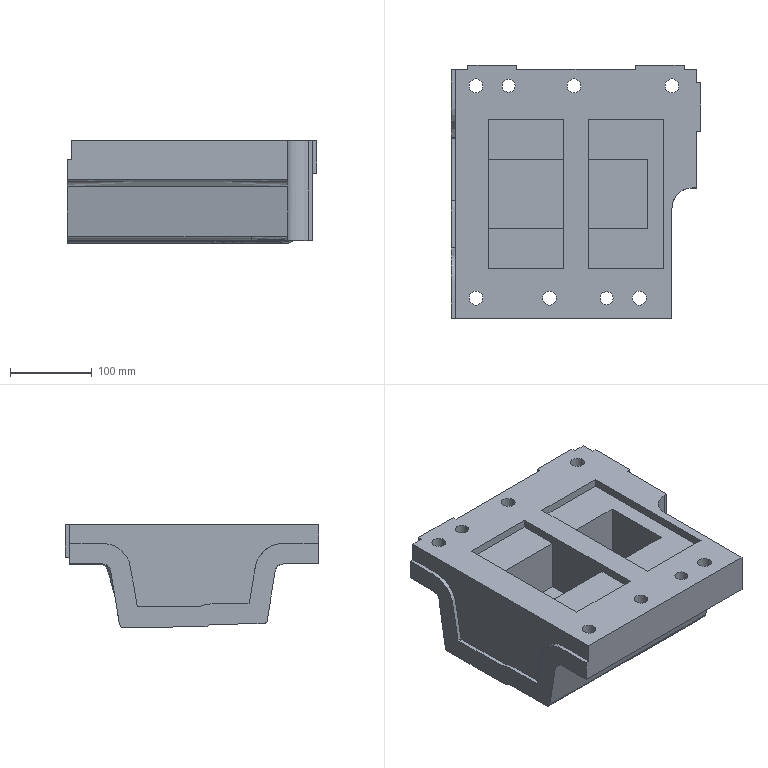Part | NX | features solid 2 | 1 solid | 155 faces | box 305 x 310 x 125.996 mm | volume 6792553 mm3 | plane 64 | spline 62 | cylinder 29 | commonest cylinder face diameters 17 x6 26 x6 12 x4 9 x3 10 x3 16 x2